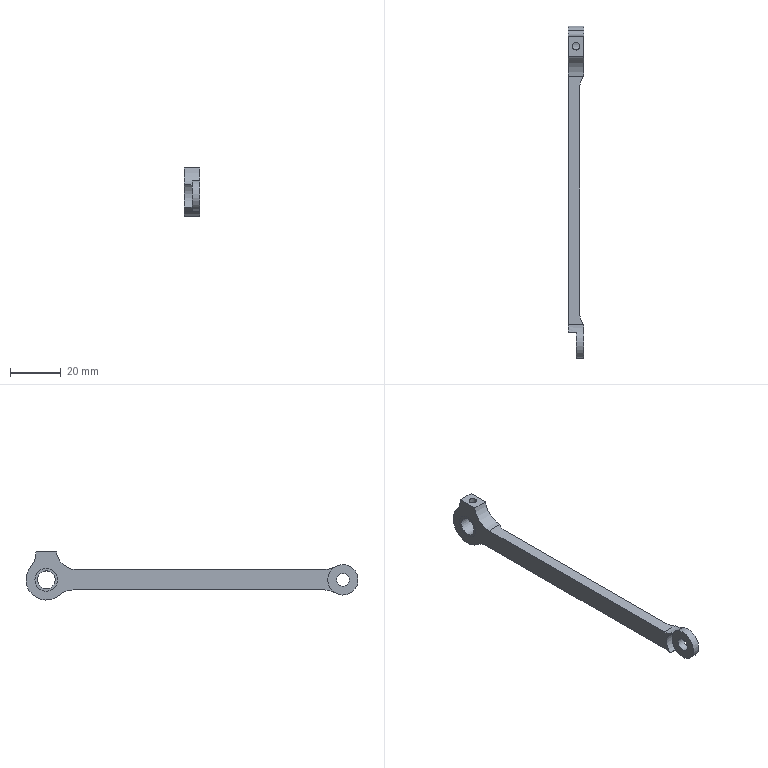Part | STEP file | 2-05.2 | 2 solids | 28 faces | box 6 x 131 x 19 mm | volume 5279 mm3 | cylinder 16 | plane 12 | commonest cylinder face diameters 16 x5 12 x4 3 x2 9 x2 5 x1 7 x1